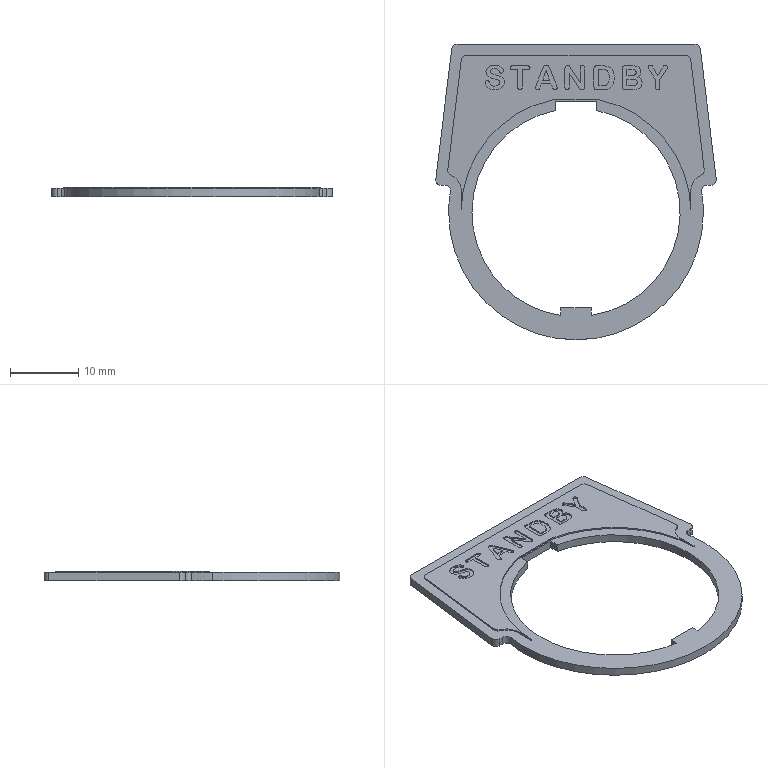Part | STEP file | Legend Standby | 1 solid | 167 faces | box 41.068 x 43.269 x 1.43 mm | volume 1005 mm3 | plane 71 | spline 70 | cylinder 26 | commonest cylinder face diameters 1.587 x15 4.763 x3 30.467 x3 37.275 x3 33.642 x2